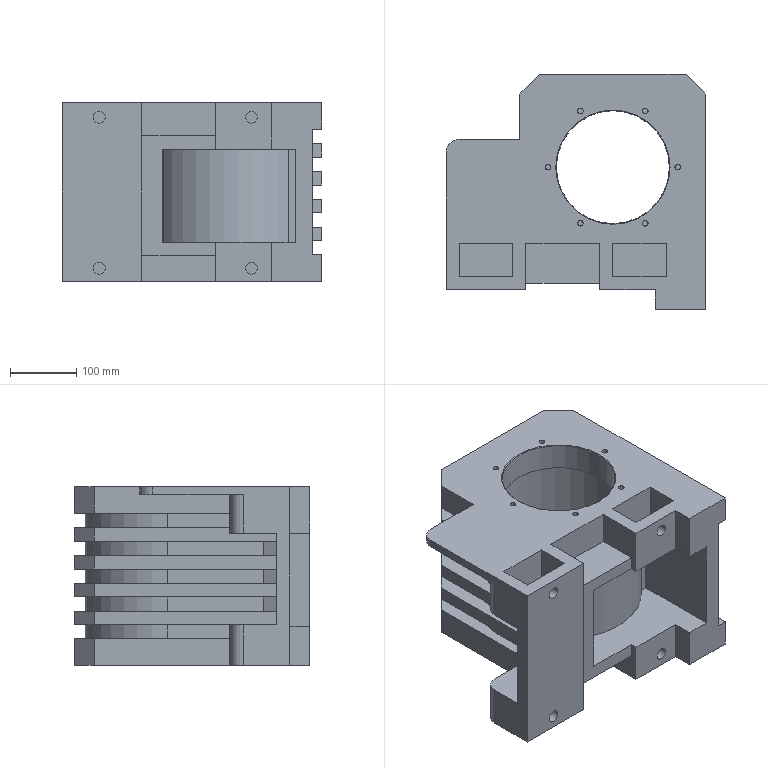Part | STEP file | 400v80 Headstock | 1 solid | 195 faces | box 391 x 354.196 x 269 mm | volume 11825762 mm3 | plane 110 | cylinder 57 | cone 28 | commonest cylinder face diameters 6.8 x12 8 x12 8.5 x12 18 x8 250 x5 40 x3